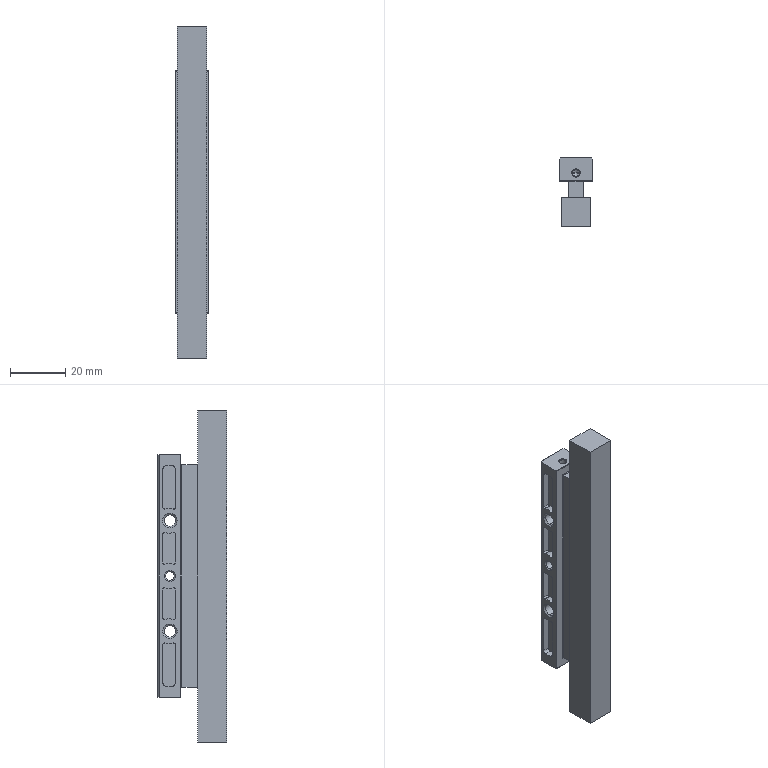Part | SolidWorks | features BaseBody 1 | 1 solid | 142 faces | box 12 x 25 x 120 mm | volume 23064 mm3 | cylinder 76 | plane 50 | cone 16 | commonest cylinder face diameters 1 x36 9 x18 2 x8 0.6 x4 4.2 x4 0.4 x2